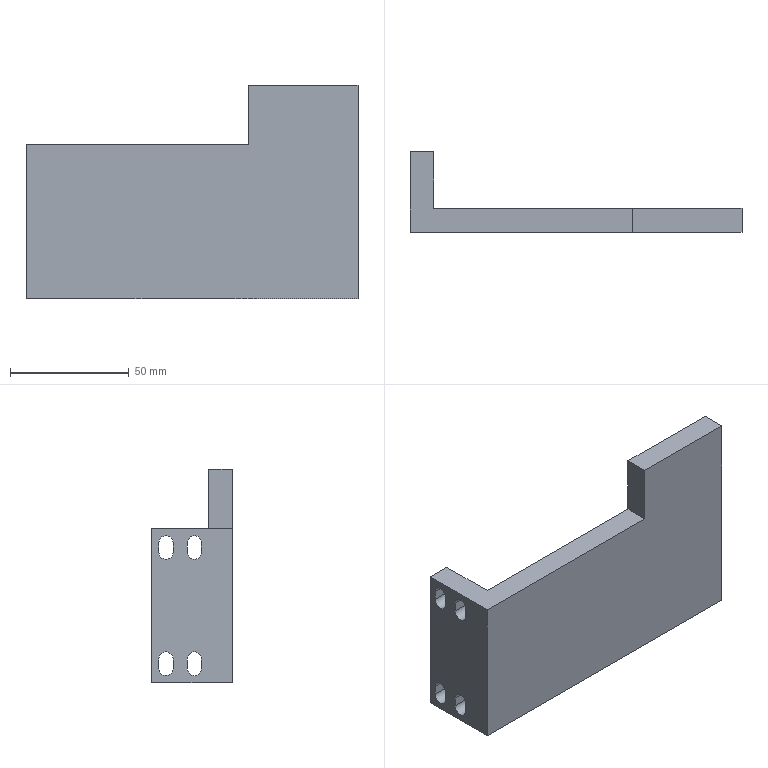Part | SolidWorks | features ICE 2, Extrusion 1 | 1 solid | 26 faces | box 140 x 34 x 90 mm | volume 116009 mm3 | plane 18 | cylinder 8 | commonest cylinder face diameters 6 x8
STEP:
#1=CARTESIAN_POINT('',(0.,0.,-32.5));
#2=VERTEX_POINT('',#1);
#3=CARTESIAN_POINT('',(140.,0.,-32.5));
#4=VERTEX_POINT('',#3);
#5=CARTESIAN_POINT('',(140.,0.,-32.5));
#6=DIRECTION('',(1.,0.,0.));
#7=VECTOR('',#6,1000.);
#8=LINE('',#5,#7);
#9=EDGE_CURVE('',#2,#4,#8,.T.);
#10=ORIENTED_EDGE('',*,*,#9,.T.);
#11=CARTESIAN_POINT('',(140.,0.,57.5));
#12=VERTEX_POINT('',#11);
#13=CARTESIAN_POINT('',(140.,0.,32.5));
#14=DIRECTION('',(0.,0.,-1.));
#15=VECTOR('',#14,1000.);
#16=LINE('',#13,#15);
#17=EDGE_CURVE('',#12,#4,#16,.T.);
#18=ORIENTED_EDGE('',*,*,#17,.F.);
#19=CARTESIAN_POINT('',(94.,0.,57.5));
#20=VERTEX_POINT('',#19);
#21=CARTESIAN_POINT('',(140.,0.,57.5));
#22=DIRECTION('',(-1.,0.,0.));
#23=VECTOR('',#22,1000.);
#24=LINE('',#21,#23);
#25=EDGE_CURVE('',#12,#20,#24,.T.);
#26=ORIENTED_EDGE('',*,*,#25,.T.);
#27=CARTESIAN_POINT('',(94.,0.,32.5));
#28=VERTEX_POINT('',#27);
#29=CARTESIAN_POINT('',(94.,0.,57.5));
#30=DIRECTION('',(0.,0.,-1.));
#31=VECTOR('',#30,1000.);
#32=LINE('',#29,#31);
#33=EDGE_CURVE('',#20,#28,#32,.T.);
#34=ORIENTED_EDGE('',*,*,#33,.T.);
#35=CARTESIAN_POINT('',(0.,0.,32.5));
#36=VERTEX_POINT('',#35);
#37=CARTESIAN_POINT('',(140.,0.,32.5));
#38=DIRECTION('',(1.,0.,0.));
#39=VECTOR('',#38,1000.);
#40=LINE('',#37,#39);
#41=EDGE_CURVE('',#36,#28,#40,.T.);
#42=ORIENTED_EDGE('',*,*,#41,.F.);
#43=CARTESIAN_POINT('',(0.,0.,32.5));
#44=DIRECTION('',(0.,0.,-1.));
#45=VECTOR('',#44,1000.);
#46=LINE('',#43,#45);
#47=EDGE_CURVE('',#36,#2,#46,.T.);
#48=ORIENTED_EDGE('',*,*,#47,.T.);
#49=EDGE_LOOP('',(#10,#18,#26,#34,#42,#48));
#50=FACE_OUTER_BOUND('',#49,.T.);
#51=CARTESIAN_POINT('',(140.,0.,32.5));
#52=DIRECTION('',(0.,1.,0.));
#53=DIRECTION('',(-1.,0.,0.));
#54=AXIS2_PLACEMENT_3D('',#51,#52,#53);
#55=PLANE('',#54);
#56=ADVANCED_FACE('',(#50),#55,.F.);
#57=CARTESIAN_POINT('',(140.,10.,-32.5));
#58=VERTEX_POINT('',#57);
#59=CARTESIAN_POINT('',(140.,10.,-32.5));
#60=DIRECTION('',(0.,1.,0.));
#61=VECTOR('',#60,1000.);
#62=LINE('',#59,#61);
#63=EDGE_CURVE('',#4,#58,#62,.T.);
#64=ORIENTED_EDGE('',*,*,#63,.T.);
#65=CARTESIAN_POINT('',(140.,10.,57.5));
#66=VERTEX_POINT('',#65);
#67=CARTESIAN_POINT('',(140.,10.,32.5));
#68=DIRECTION('',(0.,0.,-1.));
#69=VECTOR('',#68,1000.);
#70=LINE('',#67,#69);
#71=EDGE_CURVE('',#66,#58,#70,.T.);
#72=ORIENTED_EDGE('',*,*,#71,.F.);
#73=CARTESIAN_POINT('',(140.,-52.355,57.5));
#74=DIRECTION('',(0.,1.,0.));
#75=VECTOR('',#74,1000.);
#76=LINE('',#73,#75);
#77=EDGE_CURVE('',#12,#66,#76,.T.);
#78=ORIENTED_EDGE('',*,*,#77,.F.);
#79=ORIENTED_EDGE('',*,*,#17,.T.);
#80=EDGE_LOOP('',(#64,#72,#78,#79));
#81=FACE_OUTER_BOUND('',#80,.T.);
#82=CARTESIAN_POINT('',(140.,10.,32.5));
#83=DIRECTION('',(-1.,0.,0.));
#84=DIRECTION('',(0.,0.,1.));
#85=AXIS2_PLACEMENT_3D('',#82,#83,#84);
#86=PLANE('',#85);
#87=ADVANCED_FACE('',(#81),#86,.F.);
#88=CARTESIAN_POINT('',(10.,10.,-32.5));
#89=VERTEX_POINT('',#88);
#90=CARTESIAN_POINT('',(10.,10.,-32.5));
#91=DIRECTION('',(-1.,0.,0.));
#92=VECTOR('',#91,1000.);
#93=LINE('',#90,#92);
#94=EDGE_CURVE('',#58,#89,#93,.T.);
#95=ORIENTED_EDGE('',*,*,#94,.T.);
#96=CARTESIAN_POINT('',(10.,10.,32.5));
#97=VERTEX_POINT('',#96);
#98=CARTESIAN_POINT('',(10.,10.,32.5));
#99=DIRECTION('',(0.,0.,-1.));
#100=VECTOR('',#99,1000.);
#101=LINE('',#98,#100);
#102=EDGE_CURVE('',#97,#89,#101,.T.);
#103=ORIENTED_EDGE('',*,*,#102,.F.);
#104=CARTESIAN_POINT('',(94.,10.,32.5));
#105=VERTEX_POINT('',#104);
#106=CARTESIAN_POINT('',(10.,10.,32.5));
#107=DIRECTION('',(-1.,0.,0.));
#108=VECTOR('',#107,1000.);
#109=LINE('',#106,#108);
#110=EDGE_CURVE('',#105,#97,#109,.T.);
#111=ORIENTED_EDGE('',*,*,#110,.F.);
#112=CARTESIAN_POINT('',(94.,10.,57.5));
#113=VERTEX_POINT('',#112);
#114=CARTESIAN_POINT('',(94.,10.,57.5));
#115=DIRECTION('',(0.,0.,1.));
#116=VECTOR('',#115,1000.);
#117=LINE('',#114,#116);
#118=EDGE_CURVE('',#105,#113,#117,.T.);
#119=ORIENTED_EDGE('',*,*,#118,.T.);
#120=CARTESIAN_POINT('',(140.,10.,57.5));
#121=DIRECTION('',(1.,0.,0.));
#122=VECTOR('',#121,1000.);
#123=LINE('',#120,#122);
#124=EDGE_CURVE('',#113,#66,#123,.T.);
#125=ORIENTED_EDGE('',*,*,#124,.T.);
#126=ORIENTED_EDGE('',*,*,#71,.T.);
#127=EDGE_LOOP('',(#95,#103,#111,#119,#125,#126));
#128=FACE_OUTER_BOUND('',#127,.T.);
#129=CARTESIAN_POINT('',(10.,10.,32.5));
#130=DIRECTION('',(0.,-1.,0.));
#131=DIRECTION('',(1.,0.,0.));
#132=AXIS2_PLACEMENT_3D('',#129,#130,#131);
#133=PLANE('',#132);
#134=ADVANCED_FACE('',(#128),#133,.F.);
#135=CARTESIAN_POINT('',(10.,25.,-22.5));
#136=VERTEX_POINT('',#135);
#137=CARTESIAN_POINT('',(10.,25.,-26.5));
#138=VERTEX_POINT('',#137);
#139=CARTESIAN_POINT('',(10.,25.,-22.5));
#140=DIRECTION('',(0.,0.,-1.));
#141=VECTOR('',#140,1000.);
#142=LINE('',#139,#141);
#143=EDGE_CURVE('',#136,#138,#142,.T.);
#144=ORIENTED_EDGE('',*,*,#143,.F.);
#145=CARTESIAN_POINT('',(10.,31.,-22.5));
#146=VERTEX_POINT('',#145);
#147=CARTESIAN_POINT('',(10.,28.,-22.5));
#148=DIRECTION('',(1.,0.,0.));
#149=DIRECTION('',(0.,1.,0.));
#150=AXIS2_PLACEMENT_3D('',#147,#148,#149);
#151=CIRCLE('',#150,3.);
#152=EDGE_CURVE('',#146,#136,#151,.T.);
#153=ORIENTED_EDGE('',*,*,#152,.F.);
#154=CARTESIAN_POINT('',(10.,31.,-26.5));
#155=VERTEX_POINT('',#154);
#156=CARTESIAN_POINT('',(10.,31.,-22.5));
#157=DIRECTION('',(0.,0.,1.));
#158=VECTOR('',#157,1000.);
#159=LINE('',#156,#158);
#160=EDGE_CURVE('',#155,#146,#159,.T.);
#161=ORIENTED_EDGE('',*,*,#160,.F.);
#162=CARTESIAN_POINT('',(10.,28.,-26.5));
#163=DIRECTION('',(1.,0.,0.));
#164=DIRECTION('',(0.,1.,0.));
#165=AXIS2_PLACEMENT_3D('',#162,#163,#164);
#166=CIRCLE('',#165,3.);
#167=EDGE_CURVE('',#138,#155,#166,.T.);
#168=ORIENTED_EDGE('',*,*,#167,.F.);
#169=EDGE_LOOP('',(#144,#153,#161,#168));
#170=FACE_BOUND('',#169,.T.);
#171=CARTESIAN_POINT('',(10.,13.,26.5));
#172=VERTEX_POINT('',#171);
#173=CARTESIAN_POINT('',(10.,13.,22.5));
#174=VERTEX_POINT('',#173);
#175=CARTESIAN_POINT('',(10.,13.,26.5));
#176=DIRECTION('',(0.,0.,-1.));
#177=VECTOR('',#176,1000.);
#178=LINE('',#175,#177);
#179=EDGE_CURVE('',#172,#174,#178,.T.);
#180=ORIENTED_EDGE('',*,*,#179,.F.);
#181=CARTESIAN_POINT('',(10.,19.,26.5));
#182=VERTEX_POINT('',#181);
#183=CARTESIAN_POINT('',(10.,16.,26.5));
#184=DIRECTION('',(1.,0.,0.));
#185=DIRECTION('',(0.,-1.,0.));
#186=AXIS2_PLACEMENT_3D('',#183,#184,#185);
#187=CIRCLE('',#186,3.);
#188=EDGE_CURVE('',#182,#172,#187,.T.);
#189=ORIENTED_EDGE('',*,*,#188,.F.);
#190=CARTESIAN_POINT('',(10.,19.,22.5));
#191=VERTEX_POINT('',#190);
#192=CARTESIAN_POINT('',(10.,19.,26.5));
#193=DIRECTION('',(0.,0.,1.));
#194=VECTOR('',#193,1000.);
#195=LINE('',#192,#194);
#196=EDGE_CURVE('',#191,#182,#195,.T.);
#197=ORIENTED_EDGE('',*,*,#196,.F.);
#198=CARTESIAN_POINT('',(10.,16.,22.5));
#199=DIRECTION('',(1.,0.,0.));
#200=DIRECTION('',(0.,-1.,0.));
#201=AXIS2_PLACEMENT_3D('',#198,#199,#200);
#202=CIRCLE('',#201,3.);
#203=EDGE_CURVE('',#174,#191,#202,.T.);
#204=ORIENTED_EDGE('',*,*,#203,.F.);
#205=EDGE_LOOP('',(#180,#189,#197,#204));
#206=FACE_BOUND('',#205,.T.);
#207=CARTESIAN_POINT('',(10.,13.,-22.5));
#208=VERTEX_POINT('',#207);
#209=CARTESIAN_POINT('',(10.,13.,-26.5));
#210=VERTEX_POINT('',#209);
#211=CARTESIAN_POINT('',(10.,13.,-22.5));
#212=DIRECTION('',(0.,0.,-1.));
#213=VECTOR('',#212,1000.);
#214=LINE('',#211,#213);
#215=EDGE_CURVE('',#208,#210,#214,.T.);
#216=ORIENTED_EDGE('',*,*,#215,.F.);
#217=CARTESIAN_POINT('',(10.,19.,-22.5));
#218=VERTEX_POINT('',#217);
#219=CARTESIAN_POINT('',(10.,16.,-22.5));
#220=DIRECTION('',(1.,0.,0.));
#221=DIRECTION('',(0.,-1.,0.));
#222=AXIS2_PLACEMENT_3D('',#219,#220,#221);
#223=CIRCLE('',#222,3.);
#224=EDGE_CURVE('',#218,#208,#223,.T.);
#225=ORIENTED_EDGE('',*,*,#224,.F.);
#226=CARTESIAN_POINT('',(10.,19.,-26.5));
#227=VERTEX_POINT('',#226);
#228=CARTESIAN_POINT('',(10.,19.,-22.5));
#229=DIRECTION('',(0.,0.,1.));
#230=VECTOR('',#229,1000.);
#231=LINE('',#228,#230);
#232=EDGE_CURVE('',#227,#218,#231,.T.);
#233=ORIENTED_EDGE('',*,*,#232,.F.);
#234=CARTESIAN_POINT('',(10.,16.,-26.5));
#235=DIRECTION('',(1.,0.,0.));
#236=DIRECTION('',(0.,-1.,0.));
#237=AXIS2_PLACEMENT_3D('',#234,#235,#236);
#238=CIRCLE('',#237,3.);
#239=EDGE_CURVE('',#210,#227,#238,.T.);
#240=ORIENTED_EDGE('',*,*,#239,.F.);
#241=EDGE_LOOP('',(#216,#225,#233,#240));
#242=FACE_BOUND('',#241,.T.);
#243=CARTESIAN_POINT('',(10.,25.,26.5));
#244=VERTEX_POINT('',#243);
#245=CARTESIAN_POINT('',(10.,25.,22.5));
#246=VERTEX_POINT('',#245);
#247=CARTESIAN_POINT('',(10.,25.,26.5));
#248=DIRECTION('',(0.,0.,-1.));
#249=VECTOR('',#248,1000.);
#250=LINE('',#247,#249);
#251=EDGE_CURVE('',#244,#246,#250,.T.);
#252=ORIENTED_EDGE('',*,*,#251,.F.);
#253=CARTESIAN_POINT('',(10.,31.,26.5));
#254=VERTEX_POINT('',#253);
#255=CARTESIAN_POINT('',(10.,28.,26.5));
#256=DIRECTION('',(1.,0.,0.));
#257=DIRECTION('',(0.,1.,0.));
#258=AXIS2_PLACEMENT_3D('',#255,#256,#257);
#259=CIRCLE('',#258,3.);
#260=EDGE_CURVE('',#254,#244,#259,.T.);
#261=ORIENTED_EDGE('',*,*,#260,.F.);
#262=CARTESIAN_POINT('',(10.,31.,22.5));
#263=VERTEX_POINT('',#262);
#264=CARTESIAN_POINT('',(10.,31.,26.5));
#265=DIRECTION('',(0.,0.,1.));
#266=VECTOR('',#265,1000.);
#267=LINE('',#264,#266);
#268=EDGE_CURVE('',#263,#254,#267,.T.);
#269=ORIENTED_EDGE('',*,*,#268,.F.);
#270=CARTESIAN_POINT('',(10.,28.,22.5));
#271=DIRECTION('',(1.,0.,0.));
#272=DIRECTION('',(0.,1.,0.));
#273=AXIS2_PLACEMENT_3D('',#270,#271,#272);
#274=CIRCLE('',#273,3.);
#275=EDGE_CURVE('',#246,#263,#274,.T.);
#276=ORIENTED_EDGE('',*,*,#275,.F.);
#277=EDGE_LOOP('',(#252,#261,#269,#276));
#278=FACE_BOUND('',#277,.T.);
#279=CARTESIAN_POINT('',(10.,34.,-32.5));
#280=VERTEX_POINT('',#279);
#281=CARTESIAN_POINT('',(10.,34.,-32.5));
#282=DIRECTION('',(0.,1.,0.));
#283=VECTOR('',#282,1000.);
#284=LINE('',#281,#283);
#285=EDGE_CURVE('',#89,#280,#284,.T.);
#286=ORIENTED_EDGE('',*,*,#285,.T.);
#287=CARTESIAN_POINT('',(10.,34.,32.5));
#288=VERTEX_POINT('',#287);
#289=CARTESIAN_POINT('',(10.,34.,32.5));
#290=DIRECTION('',(0.,0.,-1.));
#291=VECTOR('',#290,1000.);
#292=LINE('',#289,#291);
#293=EDGE_CURVE('',#288,#280,#292,.T.);
#294=ORIENTED_EDGE('',*,*,#293,.F.);
#295=CARTESIAN_POINT('',(10.,34.,32.5));
#296=DIRECTION('',(0.,1.,0.));
#297=VECTOR('',#296,1000.);
#298=LINE('',#295,#297);
#299=EDGE_CURVE('',#97,#288,#298,.T.);
#300=ORIENTED_EDGE('',*,*,#299,.F.);
#301=ORIENTED_EDGE('',*,*,#102,.T.);
#302=EDGE_LOOP('',(#286,#294,#300,#301));
#303=FACE_OUTER_BOUND('',#302,.T.);
#304=CARTESIAN_POINT('',(10.,34.,32.5));
#305=DIRECTION('',(-1.,0.,0.));
#306=DIRECTION('',(0.,-1.,0.));
#307=AXIS2_PLACEMENT_3D('',#304,#305,#306);
#308=PLANE('',#307);
#309=ADVANCED_FACE('',(#170,#206,#242,#278,#303),#308,.F.);
#310=CARTESIAN_POINT('',(0.,34.,-32.5));
#311=VERTEX_POINT('',#310);
#312=CARTESIAN_POINT('',(0.,34.,-32.5));
#313=DIRECTION('',(-1.,0.,0.));
#314=VECTOR('',#313,1000.);
#315=LINE('',#312,#314);
#316=EDGE_CURVE('',#280,#311,#315,.T.);
#317=ORIENTED_EDGE('',*,*,#316,.T.);
#318=CARTESIAN_POINT('',(0.,34.,32.5));
#319=VERTEX_POINT('',#318);
#320=CARTESIAN_POINT('',(0.,34.,32.5));
#321=DIRECTION('',(0.,0.,-1.));
#322=VECTOR('',#321,1000.);
#323=LINE('',#320,#322);
#324=EDGE_CURVE('',#319,#311,#323,.T.);
#325=ORIENTED_EDGE('',*,*,#324,.F.);
#326=CARTESIAN_POINT('',(0.,34.,32.5));
#327=DIRECTION('',(-1.,0.,0.));
#328=VECTOR('',#327,1000.);
#329=LINE('',#326,#328);
#330=EDGE_CURVE('',#288,#319,#329,.T.);
#331=ORIENTED_EDGE('',*,*,#330,.F.);
#332=ORIENTED_EDGE('',*,*,#293,.T.);
#333=EDGE_LOOP('',(#317,#325,#331,#332));
#334=FACE_OUTER_BOUND('',#333,.T.);
#335=CARTESIAN_POINT('',(0.,34.,32.5));
#336=DIRECTION('',(0.,-1.,0.));
#337=DIRECTION('',(0.,0.,-1.));
#338=AXIS2_PLACEMENT_3D('',#335,#336,#337);
#339=PLANE('',#338);
#340=ADVANCED_FACE('',(#334),#339,.F.);
#341=CARTESIAN_POINT('',(0.,31.,-22.5));
#342=VERTEX_POINT('',#341);
#343=CARTESIAN_POINT('',(0.,31.,-26.5));
#344=VERTEX_POINT('',#343);
#345=CARTESIAN_POINT('',(0.,31.,-22.5));
#346=DIRECTION('',(0.,0.,-1.));
#347=VECTOR('',#346,1000.);
#348=LINE('',#345,#347);
#349=EDGE_CURVE('',#342,#344,#348,.T.);
#350=ORIENTED_EDGE('',*,*,#349,.F.);
#351=CARTESIAN_POINT('',(0.,25.,-22.5));
#352=VERTEX_POINT('',#351);
#353=CARTESIAN_POINT('',(0.,28.,-22.5));
#354=DIRECTION('',(-1.,0.,0.));
#355=DIRECTION('',(0.,1.,0.));
#356=AXIS2_PLACEMENT_3D('',#353,#354,#355);
#357=CIRCLE('',#356,3.);
#358=EDGE_CURVE('',#352,#342,#357,.T.);
#359=ORIENTED_EDGE('',*,*,#358,.F.);
#360=CARTESIAN_POINT('',(0.,25.,-26.5));
#361=VERTEX_POINT('',#360);
#362=CARTESIAN_POINT('',(0.,25.,-22.5));
#363=DIRECTION('',(0.,0.,1.));
#364=VECTOR('',#363,1000.);
#365=LINE('',#362,#364);
#366=EDGE_CURVE('',#361,#352,#365,.T.);
#367=ORIENTED_EDGE('',*,*,#366,.F.);
#368=CARTESIAN_POINT('',(0.,28.,-26.5));
#369=DIRECTION('',(-1.,0.,0.));
#370=DIRECTION('',(0.,1.,0.));
#371=AXIS2_PLACEMENT_3D('',#368,#369,#370);
#372=CIRCLE('',#371,3.);
#373=EDGE_CURVE('',#344,#361,#372,.T.);
#374=ORIENTED_EDGE('',*,*,#373,.F.);
#375=EDGE_LOOP('',(#350,#359,#367,#374));
#376=FACE_BOUND('',#375,.T.);
#377=CARTESIAN_POINT('',(0.,19.,26.5));
#378=VERTEX_POINT('',#377);
#379=CARTESIAN_POINT('',(0.,19.,22.5));
#380=VERTEX_POINT('',#379);
#381=CARTESIAN_POINT('',(0.,19.,26.5));
#382=DIRECTION('',(0.,0.,-1.));
#383=VECTOR('',#382,1000.);
#384=LINE('',#381,#383);
#385=EDGE_CURVE('',#378,#380,#384,.T.);
#386=ORIENTED_EDGE('',*,*,#385,.F.);
#387=CARTESIAN_POINT('',(0.,13.,26.5));
#388=VERTEX_POINT('',#387);
#389=CARTESIAN_POINT('',(0.,16.,26.5));
#390=DIRECTION('',(-1.,0.,0.));
#391=DIRECTION('',(0.,1.,0.));
#392=AXIS2_PLACEMENT_3D('',#389,#390,#391);
#393=CIRCLE('',#392,3.);
#394=EDGE_CURVE('',#388,#378,#393,.T.);
#395=ORIENTED_EDGE('',*,*,#394,.F.);
#396=CARTESIAN_POINT('',(0.,13.,22.5));
#397=VERTEX_POINT('',#396);
#398=CARTESIAN_POINT('',(0.,13.,26.5));
#399=DIRECTION('',(0.,0.,1.));
#400=VECTOR('',#399,1000.);
#401=LINE('',#398,#400);
#402=EDGE_CURVE('',#397,#388,#401,.T.);
#403=ORIENTED_EDGE('',*,*,#402,.F.);
#404=CARTESIAN_POINT('',(0.,16.,22.5));
#405=DIRECTION('',(-1.,0.,0.));
#406=DIRECTION('',(0.,1.,0.));
#407=AXIS2_PLACEMENT_3D('',#404,#405,#406);
#408=CIRCLE('',#407,3.);
#409=EDGE_CURVE('',#380,#397,#408,.T.);
#410=ORIENTED_EDGE('',*,*,#409,.F.);
#411=EDGE_LOOP('',(#386,#395,#403,#410));
#412=FACE_BOUND('',#411,.T.);
#413=CARTESIAN_POINT('',(0.,19.,-22.5));
#414=VERTEX_POINT('',#413);
#415=CARTESIAN_POINT('',(0.,19.,-26.5));
#416=VERTEX_POINT('',#415);
#417=CARTESIAN_POINT('',(0.,19.,-22.5));
#418=DIRECTION('',(0.,0.,-1.));
#419=VECTOR('',#418,1000.);
#420=LINE('',#417,#419);
#421=EDGE_CURVE('',#414,#416,#420,.T.);
#422=ORIENTED_EDGE('',*,*,#421,.F.);
#423=CARTESIAN_POINT('',(0.,13.,-22.5));
#424=VERTEX_POINT('',#423);
#425=CARTESIAN_POINT('',(0.,16.,-22.5));
#426=DIRECTION('',(-1.,0.,0.));
#427=DIRECTION('',(0.,1.,0.));
#428=AXIS2_PLACEMENT_3D('',#425,#426,#427);
#429=CIRCLE('',#428,3.);
#430=EDGE_CURVE('',#424,#414,#429,.T.);
#431=ORIENTED_EDGE('',*,*,#430,.F.);
#432=CARTESIAN_POINT('',(0.,13.,-26.5));
#433=VERTEX_POINT('',#432);
#434=CARTESIAN_POINT('',(0.,13.,-22.5));
#435=DIRECTION('',(0.,0.,1.));
#436=VECTOR('',#435,1000.);
#437=LINE('',#434,#436);
#438=EDGE_CURVE('',#433,#424,#437,.T.);
#439=ORIENTED_EDGE('',*,*,#438,.F.);
#440=CARTESIAN_POINT('',(0.,16.,-26.5));
#441=DIRECTION('',(-1.,0.,0.));
#442=DIRECTION('',(0.,1.,0.));
#443=AXIS2_PLACEMENT_3D('',#440,#441,#442);
#444=CIRCLE('',#443,3.);
#445=EDGE_CURVE('',#416,#433,#444,.T.);
#446=ORIENTED_EDGE('',*,*,#445,.F.);
#447=EDGE_LOOP('',(#422,#431,#439,#446));
#448=FACE_BOUND('',#447,.T.);
#449=CARTESIAN_POINT('',(0.,31.,26.5));
#450=VERTEX_POINT('',#449);
#451=CARTESIAN_POINT('',(0.,31.,22.5));
#452=VERTEX_POINT('',#451);
#453=CARTESIAN_POINT('',(0.,31.,26.5));
#454=DIRECTION('',(0.,0.,-1.));
#455=VECTOR('',#454,1000.);
#456=LINE('',#453,#455);
#457=EDGE_CURVE('',#450,#452,#456,.T.);
#458=ORIENTED_EDGE('',*,*,#457,.F.);
#459=CARTESIAN_POINT('',(0.,25.,26.5));
#460=VERTEX_POINT('',#459);
#461=CARTESIAN_POINT('',(0.,28.,26.5));
#462=DIRECTION('',(-1.,0.,0.));
#463=DIRECTION('',(0.,1.,0.));
#464=AXIS2_PLACEMENT_3D('',#461,#462,#463);
#465=CIRCLE('',#464,3.);
#466=EDGE_CURVE('',#460,#450,#465,.T.);
#467=ORIENTED_EDGE('',*,*,#466,.F.);
#468=CARTESIAN_POINT('',(0.,25.,22.5));
#469=VERTEX_POINT('',#468);
#470=CARTESIAN_POINT('',(0.,25.,26.5));
#471=DIRECTION('',(0.,0.,1.));
#472=VECTOR('',#471,1000.);
#473=LINE('',#470,#472);
#474=EDGE_CURVE('',#469,#460,#473,.T.);
#475=ORIENTED_EDGE('',*,*,#474,.F.);
#476=CARTESIAN_POINT('',(0.,28.,22.5));
#477=DIRECTION('',(-1.,0.,0.));
#478=DIRECTION('',(0.,1.,0.));
#479=AXIS2_PLACEMENT_3D('',#476,#477,#478);
#480=CIRCLE('',#479,3.);
#481=EDGE_CURVE('',#452,#469,#480,.T.);
#482=ORIENTED_EDGE('',*,*,#481,.F.);
#483=EDGE_LOOP('',(#458,#467,#475,#482));
#484=FACE_BOUND('',#483,.T.);
#485=CARTESIAN_POINT('',(0.,0.,-32.5));
#486=DIRECTION('',(0.,-1.,0.));
#487=VECTOR('',#486,1000.);
#488=LINE('',#485,#487);
#489=EDGE_CURVE('',#311,#2,#488,.T.);
#490=ORIENTED_EDGE('',*,*,#489,.T.);
#491=ORIENTED_EDGE('',*,*,#47,.F.);
#492=CARTESIAN_POINT('',(0.,0.,32.5));
#493=DIRECTION('',(0.,-1.,0.));
#494=VECTOR('',#493,1000.);
#495=LINE('',#492,#494);
#496=EDGE_CURVE('',#319,#36,#495,.T.);
#497=ORIENTED_EDGE('',*,*,#496,.F.);
#498=ORIENTED_EDGE('',*,*,#324,.T.);
#499=EDGE_LOOP('',(#490,#491,#497,#498));
#500=FACE_OUTER_BOUND('',#499,.T.);
#501=CARTESIAN_POINT('',(0.,0.,32.5));
#502=DIRECTION('',(1.,0.,0.));
#503=DIRECTION('',(0.,1.,0.));
#504=AXIS2_PLACEMENT_3D('',#501,#502,#503);
#505=PLANE('',#504);
#506=ADVANCED_FACE('',(#376,#412,#448,#484,#500),#505,.F.);
#507=ORIENTED_EDGE('',*,*,#41,.T.);
#508=CARTESIAN_POINT('',(94.,-52.355,32.5));
#509=DIRECTION('',(0.,1.,0.));
#510=VECTOR('',#509,1000.);
#511=LINE('',#508,#510);
#512=EDGE_CURVE('',#28,#105,#511,.T.);
#513=ORIENTED_EDGE('',*,*,#512,.T.);
#514=ORIENTED_EDGE('',*,*,#110,.T.);
#515=ORIENTED_EDGE('',*,*,#299,.T.);
#516=ORIENTED_EDGE('',*,*,#330,.T.);
#517=ORIENTED_EDGE('',*,*,#496,.T.);
#518=EDGE_LOOP('',(#507,#513,#514,#515,#516,#517));
#519=FACE_OUTER_BOUND('',#518,.T.);
#520=CARTESIAN_POINT('',(0.,0.,32.5));
#521=DIRECTION('',(0.,0.,-1.));
#522=DIRECTION('',(-1.,0.,0.));
#523=AXIS2_PLACEMENT_3D('',#520,#521,#522);
#524=PLANE('',#523);
#525=ADVANCED_FACE('',(#519),#524,.F.);
#526=ORIENTED_EDGE('',*,*,#9,.F.);
#527=ORIENTED_EDGE('',*,*,#489,.F.);
#528=ORIENTED_EDGE('',*,*,#316,.F.);
#529=ORIENTED_EDGE('',*,*,#285,.F.);
#530=ORIENTED_EDGE('',*,*,#94,.F.);
#531=ORIENTED_EDGE('',*,*,#63,.F.);
#532=EDGE_LOOP('',(#526,#527,#528,#529,#530,#531));
#533=FACE_OUTER_BOUND('',#532,.T.);
#534=CARTESIAN_POINT('',(0.,0.,-32.5));
#535=DIRECTION('',(0.,0.,-1.));
#536=DIRECTION('',(-1.,0.,0.));
#537=AXIS2_PLACEMENT_3D('',#534,#535,#536);
#538=PLANE('',#537);
#539=ADVANCED_FACE('',(#533),#538,.T.);
#540=ORIENTED_EDGE('',*,*,#466,.T.);
#541=CARTESIAN_POINT('',(-0.001,31.,26.5));
#542=DIRECTION('',(1.,0.,0.));
#543=VECTOR('',#542,1000.);
#544=LINE('',#541,#543);
#545=EDGE_CURVE('',#450,#254,#544,.T.);
#546=ORIENTED_EDGE('',*,*,#545,.T.);
#547=ORIENTED_EDGE('',*,*,#260,.T.);
#548=CARTESIAN_POINT('',(-0.001,25.,26.5));
#549=DIRECTION('',(1.,0.,0.));
#550=VECTOR('',#549,1000.);
#551=LINE('',#548,#550);
#552=EDGE_CURVE('',#460,#244,#551,.T.);
#553=ORIENTED_EDGE('',*,*,#552,.F.);
#554=EDGE_LOOP('',(#540,#546,#547,#553));
#555=FACE_OUTER_BOUND('',#554,.T.);
#556=CARTESIAN_POINT('',(-0.001,28.,26.5));
#557=DIRECTION('',(1.,0.,0.));
#558=DIRECTION('',(0.,1.,0.));
#559=AXIS2_PLACEMENT_3D('',#556,#557,#558);
#560=CYLINDRICAL_SURFACE('',#559,3.);
#561=ADVANCED_FACE('',(#555),#560,.F.);
#562=ORIENTED_EDGE('',*,*,#457,.T.);
#563=CARTESIAN_POINT('',(-0.001,31.,22.5));
#564=DIRECTION('',(1.,0.,0.));
#565=VECTOR('',#564,1000.);
#566=LINE('',#563,#565);
#567=EDGE_CURVE('',#452,#263,#566,.T.);
#568=ORIENTED_EDGE('',*,*,#567,.T.);
#569=ORIENTED_EDGE('',*,*,#268,.T.);
#570=ORIENTED_EDGE('',*,*,#545,.F.);
#571=EDGE_LOOP('',(#562,#568,#569,#570));
#572=FACE_OUTER_BOUND('',#571,.T.);
#573=CARTESIAN_POINT('',(-0.001,31.,26.5));
#574=DIRECTION('',(0.,1.,0.));
#575=DIRECTION('',(-1.,0.,0.));
#576=AXIS2_PLACEMENT_3D('',#573,#574,#575);
#577=PLANE('',#576);
#578=ADVANCED_FACE('',(#572),#577,.F.);
#579=ORIENTED_EDGE('',*,*,#481,.T.);
#580=CARTESIAN_POINT('',(-0.001,25.,22.5));
#581=DIRECTION('',(1.,0.,0.));
#582=VECTOR('',#581,1000.);
#583=LINE('',#580,#582);
#584=EDGE_CURVE('',#469,#246,#583,.T.);
#585=ORIENTED_EDGE('',*,*,#584,.T.);
#586=ORIENTED_EDGE('',*,*,#275,.T.);
#587=ORIENTED_EDGE('',*,*,#567,.F.);
#588=EDGE_LOOP('',(#579,#585,#586,#587));
#589=FACE_OUTER_BOUND('',#588,.T.);
#590=CARTESIAN_POINT('',(-0.001,28.,22.5));
#591=DIRECTION('',(1.,0.,0.));
#592=DIRECTION('',(0.,1.,0.));
#593=AXIS2_PLACEMENT_3D('',#590,#591,#592);
#594=CYLINDRICAL_SURFACE('',#593,3.);
#595=ADVANCED_FACE('',(#589),#594,.F.);
#596=ORIENTED_EDGE('',*,*,#474,.T.);
#597=ORIENTED_EDGE('',*,*,#552,.T.);
#598=ORIENTED_EDGE('',*,*,#251,.T.);
#599=ORIENTED_EDGE('',*,*,#584,.F.);
#600=EDGE_LOOP('',(#596,#597,#598,#599));
#601=FACE_OUTER_BOUND('',#600,.T.);
#602=CARTESIAN_POINT('',(-0.001,25.,26.5));
#603=DIRECTION('',(0.,-1.,0.));
#604=DIRECTION('',(1.,0.,0.));
#605=AXIS2_PLACEMENT_3D('',#602,#603,#604);
#606=PLANE('',#605);
#607=ADVANCED_FACE('',(#601),#606,.F.);
#608=ORIENTED_EDGE('',*,*,#430,.T.);
#609=CARTESIAN_POINT('',(-0.001,19.,-22.5));
#610=DIRECTION('',(1.,0.,0.));
#611=VECTOR('',#610,1000.);
#612=LINE('',#609,#611);
#613=EDGE_CURVE('',#414,#218,#612,.T.);
#614=ORIENTED_EDGE('',*,*,#613,.T.);
#615=ORIENTED_EDGE('',*,*,#224,.T.);
#616=CARTESIAN_POINT('',(-0.001,13.,-22.5));
#617=DIRECTION('',(1.,0.,0.));
#618=VECTOR('',#617,1000.);
#619=LINE('',#616,#618);
#620=EDGE_CURVE('',#424,#208,#619,.T.);
#621=ORIENTED_EDGE('',*,*,#620,.F.);
#622=EDGE_LOOP('',(#608,#614,#615,#621));
#623=FACE_OUTER_BOUND('',#622,.T.);
#624=CARTESIAN_POINT('',(-0.001,16.,-22.5));
#625=DIRECTION('',(1.,0.,0.));
#626=DIRECTION('',(0.,1.,0.));
#627=AXIS2_PLACEMENT_3D('',#624,#625,#626);
#628=CYLINDRICAL_SURFACE('',#627,3.);
#629=ADVANCED_FACE('',(#623),#628,.F.);
#630=ORIENTED_EDGE('',*,*,#421,.T.);
#631=CARTESIAN_POINT('',(-0.001,19.,-26.5));
#632=DIRECTION('',(1.,0.,0.));
#633=VECTOR('',#632,1000.);
#634=LINE('',#631,#633);
#635=EDGE_CURVE('',#416,#227,#634,.T.);
#636=ORIENTED_EDGE('',*,*,#635,.T.);
#637=ORIENTED_EDGE('',*,*,#232,.T.);
#638=ORIENTED_EDGE('',*,*,#613,.F.);
#639=EDGE_LOOP('',(#630,#636,#637,#638));
#640=FACE_OUTER_BOUND('',#639,.T.);
#641=CARTESIAN_POINT('',(-0.001,19.,-22.5));
#642=DIRECTION('',(0.,1.,0.));
#643=DIRECTION('',(-1.,0.,0.));
#644=AXIS2_PLACEMENT_3D('',#641,#642,#643);
#645=PLANE('',#644);
#646=ADVANCED_FACE('',(#640),#645,.F.);
#647=ORIENTED_EDGE('',*,*,#445,.T.);
#648=CARTESIAN_POINT('',(-0.001,13.,-26.5));
#649=DIRECTION('',(1.,0.,0.));
#650=VECTOR('',#649,1000.);
#651=LINE('',#648,#650);
#652=EDGE_CURVE('',#433,#210,#651,.T.);
#653=ORIENTED_EDGE('',*,*,#652,.T.);
#654=ORIENTED_EDGE('',*,*,#239,.T.);
#655=ORIENTED_EDGE('',*,*,#635,.F.);
#656=EDGE_LOOP('',(#647,#653,#654,#655));
#657=FACE_OUTER_BOUND('',#656,.T.);
#658=CARTESIAN_POINT('',(-0.001,16.,-26.5));
#659=DIRECTION('',(1.,0.,0.));
#660=DIRECTION('',(0.,1.,0.));
#661=AXIS2_PLACEMENT_3D('',#658,#659,#660);
#662=CYLINDRICAL_SURFACE('',#661,3.);
#663=ADVANCED_FACE('',(#657),#662,.F.);
#664=ORIENTED_EDGE('',*,*,#438,.T.);
#665=ORIENTED_EDGE('',*,*,#620,.T.);
#666=ORIENTED_EDGE('',*,*,#215,.T.);
#667=ORIENTED_EDGE('',*,*,#652,.F.);
#668=EDGE_LOOP('',(#664,#665,#666,#667));
#669=FACE_OUTER_BOUND('',#668,.T.);
#670=CARTESIAN_POINT('',(-0.001,13.,-22.5));
#671=DIRECTION('',(0.,-1.,0.));
#672=DIRECTION('',(1.,0.,0.));
#673=AXIS2_PLACEMENT_3D('',#670,#671,#672);
#674=PLANE('',#673);
#675=ADVANCED_FACE('',(#669),#674,.F.);
#676=ORIENTED_EDGE('',*,*,#394,.T.);
#677=CARTESIAN_POINT('',(-0.001,19.,26.5));
#678=DIRECTION('',(1.,0.,0.));
#679=VECTOR('',#678,1000.);
#680=LINE('',#677,#679);
#681=EDGE_CURVE('',#378,#182,#680,.T.);
#682=ORIENTED_EDGE('',*,*,#681,.T.);
#683=ORIENTED_EDGE('',*,*,#188,.T.);
#684=CARTESIAN_POINT('',(-0.001,13.,26.5));
#685=DIRECTION('',(1.,0.,0.));
#686=VECTOR('',#685,1000.);
#687=LINE('',#684,#686);
#688=EDGE_CURVE('',#388,#172,#687,.T.);
#689=ORIENTED_EDGE('',*,*,#688,.F.);
#690=EDGE_LOOP('',(#676,#682,#683,#689));
#691=FACE_OUTER_BOUND('',#690,.T.);
#692=CARTESIAN_POINT('',(-0.001,16.,26.5));
#693=DIRECTION('',(1.,0.,0.));
#694=DIRECTION('',(0.,1.,0.));
#695=AXIS2_PLACEMENT_3D('',#692,#693,#694);
#696=CYLINDRICAL_SURFACE('',#695,3.);
#697=ADVANCED_FACE('',(#691),#696,.F.);
#698=ORIENTED_EDGE('',*,*,#385,.T.);
#699=CARTESIAN_POINT('',(-0.001,19.,22.5));
#700=DIRECTION('',(1.,0.,0.));
#701=VECTOR('',#700,1000.);
#702=LINE('',#699,#701);
#703=EDGE_CURVE('',#380,#191,#702,.T.);
#704=ORIENTED_EDGE('',*,*,#703,.T.);
#705=ORIENTED_EDGE('',*,*,#196,.T.);
#706=ORIENTED_EDGE('',*,*,#681,.F.);
#707=EDGE_LOOP('',(#698,#704,#705,#706));
#708=FACE_OUTER_BOUND('',#707,.T.);
#709=CARTESIAN_POINT('',(-0.001,19.,26.5));
#710=DIRECTION('',(0.,1.,0.));
#711=DIRECTION('',(-1.,0.,0.));
#712=AXIS2_PLACEMENT_3D('',#709,#710,#711);
#713=PLANE('',#712);
#714=ADVANCED_FACE('',(#708),#713,.F.);
#715=ORIENTED_EDGE('',*,*,#409,.T.);
#716=CARTESIAN_POINT('',(-0.001,13.,22.5));
#717=DIRECTION('',(1.,0.,0.));
#718=VECTOR('',#717,1000.);
#719=LINE('',#716,#718);
#720=EDGE_CURVE('',#397,#174,#719,.T.);
#721=ORIENTED_EDGE('',*,*,#720,.T.);
#722=ORIENTED_EDGE('',*,*,#203,.T.);
#723=ORIENTED_EDGE('',*,*,#703,.F.);
#724=EDGE_LOOP('',(#715,#721,#722,#723));
#725=FACE_OUTER_BOUND('',#724,.T.);
#726=CARTESIAN_POINT('',(-0.001,16.,22.5));
#727=DIRECTION('',(1.,0.,0.));
#728=DIRECTION('',(0.,1.,0.));
#729=AXIS2_PLACEMENT_3D('',#726,#727,#728);
#730=CYLINDRICAL_SURFACE('',#729,3.);
#731=ADVANCED_FACE('',(#725),#730,.F.);
#732=ORIENTED_EDGE('',*,*,#402,.T.);
#733=ORIENTED_EDGE('',*,*,#688,.T.);
#734=ORIENTED_EDGE('',*,*,#179,.T.);
#735=ORIENTED_EDGE('',*,*,#720,.F.);
#736=EDGE_LOOP('',(#732,#733,#734,#735));
#737=FACE_OUTER_BOUND('',#736,.T.);
#738=CARTESIAN_POINT('',(-0.001,13.,26.5));
#739=DIRECTION('',(0.,-1.,0.));
#740=DIRECTION('',(1.,0.,0.));
#741=AXIS2_PLACEMENT_3D('',#738,#739,#740);
#742=PLANE('',#741);
#743=ADVANCED_FACE('',(#737),#742,.F.);
#744=ORIENTED_EDGE('',*,*,#358,.T.);
#745=CARTESIAN_POINT('',(-0.001,31.,-22.5));
#746=DIRECTION('',(1.,0.,0.));
#747=VECTOR('',#746,1000.);
#748=LINE('',#745,#747);
#749=EDGE_CURVE('',#342,#146,#748,.T.);
#750=ORIENTED_EDGE('',*,*,#749,.T.);
#751=ORIENTED_EDGE('',*,*,#152,.T.);
#752=CARTESIAN_POINT('',(-0.001,25.,-22.5));
#753=DIRECTION('',(1.,0.,0.));
#754=VECTOR('',#753,1000.);
#755=LINE('',#752,#754);
#756=EDGE_CURVE('',#352,#136,#755,.T.);
#757=ORIENTED_EDGE('',*,*,#756,.F.);
#758=EDGE_LOOP('',(#744,#750,#751,#757));
#759=FACE_OUTER_BOUND('',#758,.T.);
#760=CARTESIAN_POINT('',(-0.001,28.,-22.5));
#761=DIRECTION('',(1.,0.,0.));
#762=DIRECTION('',(0.,1.,0.));
#763=AXIS2_PLACEMENT_3D('',#760,#761,#762);
#764=CYLINDRICAL_SURFACE('',#763,3.);
#765=ADVANCED_FACE('',(#759),#764,.F.);
#766=ORIENTED_EDGE('',*,*,#349,.T.);
#767=CARTESIAN_POINT('',(-0.001,31.,-26.5));
#768=DIRECTION('',(1.,0.,0.));
#769=VECTOR('',#768,1000.);
#770=LINE('',#767,#769);
#771=EDGE_CURVE('',#344,#155,#770,.T.);
#772=ORIENTED_EDGE('',*,*,#771,.T.);
#773=ORIENTED_EDGE('',*,*,#160,.T.);
#774=ORIENTED_EDGE('',*,*,#749,.F.);
#775=EDGE_LOOP('',(#766,#772,#773,#774));
#776=FACE_OUTER_BOUND('',#775,.T.);
#777=CARTESIAN_POINT('',(-0.001,31.,-22.5));
#778=DIRECTION('',(0.,1.,0.));
#779=DIRECTION('',(-1.,0.,0.));
#780=AXIS2_PLACEMENT_3D('',#777,#778,#779);
#781=PLANE('',#780);
#782=ADVANCED_FACE('',(#776),#781,.F.);
#783=ORIENTED_EDGE('',*,*,#373,.T.);
#784=CARTESIAN_POINT('',(-0.001,25.,-26.5));
#785=DIRECTION('',(1.,0.,0.));
#786=VECTOR('',#785,1000.);
#787=LINE('',#784,#786);
#788=EDGE_CURVE('',#361,#138,#787,.T.);
#789=ORIENTED_EDGE('',*,*,#788,.T.);
#790=ORIENTED_EDGE('',*,*,#167,.T.);
#791=ORIENTED_EDGE('',*,*,#771,.F.);
#792=EDGE_LOOP('',(#783,#789,#790,#791));
#793=FACE_OUTER_BOUND('',#792,.T.);
#794=CARTESIAN_POINT('',(-0.001,28.,-26.5));
#795=DIRECTION('',(1.,0.,0.));
#796=DIRECTION('',(0.,1.,0.));
#797=AXIS2_PLACEMENT_3D('',#794,#795,#796);
#798=CYLINDRICAL_SURFACE('',#797,3.);
#799=ADVANCED_FACE('',(#793),#798,.F.);
#800=ORIENTED_EDGE('',*,*,#366,.T.);
#801=ORIENTED_EDGE('',*,*,#756,.T.);
#802=ORIENTED_EDGE('',*,*,#143,.T.);
#803=ORIENTED_EDGE('',*,*,#788,.F.);
#804=EDGE_LOOP('',(#800,#801,#802,#803));
#805=FACE_OUTER_BOUND('',#804,.T.);
#806=CARTESIAN_POINT('',(-0.001,25.,-22.5));
#807=DIRECTION('',(0.,-1.,0.));
#808=DIRECTION('',(1.,0.,0.));
#809=AXIS2_PLACEMENT_3D('',#806,#807,#808);
#810=PLANE('',#809);
#811=ADVANCED_FACE('',(#805),#810,.F.);
#812=ORIENTED_EDGE('',*,*,#25,.F.);
#813=ORIENTED_EDGE('',*,*,#77,.T.);
#814=ORIENTED_EDGE('',*,*,#124,.F.);
#815=CARTESIAN_POINT('',(94.,-52.355,57.5));
#816=DIRECTION('',(0.,1.,0.));
#817=VECTOR('',#816,1000.);
#818=LINE('',#815,#817);
#819=EDGE_CURVE('',#20,#113,#818,.T.);
#820=ORIENTED_EDGE('',*,*,#819,.F.);
#821=EDGE_LOOP('',(#812,#813,#814,#820));
#822=FACE_OUTER_BOUND('',#821,.T.);
#823=CARTESIAN_POINT('',(140.,-52.355,57.5));
#824=DIRECTION('',(0.,0.,1.));
#825=DIRECTION('',(1.,0.,0.));
#826=AXIS2_PLACEMENT_3D('',#823,#824,#825);
#827=PLANE('',#826);
#828=ADVANCED_FACE('',(#822),#827,.T.);
#829=ORIENTED_EDGE('',*,*,#33,.F.);
#830=ORIENTED_EDGE('',*,*,#819,.T.);
#831=ORIENTED_EDGE('',*,*,#118,.F.);
#832=ORIENTED_EDGE('',*,*,#512,.F.);
#833=EDGE_LOOP('',(#829,#830,#831,#832));
#834=FACE_OUTER_BOUND('',#833,.T.);
#835=CARTESIAN_POINT('',(94.,-52.355,57.5));
#836=DIRECTION('',(-1.,0.,0.));
#837=DIRECTION('',(0.,-1.,0.));
#838=AXIS2_PLACEMENT_3D('',#835,#836,#837);
#839=PLANE('',#838);
#840=ADVANCED_FACE('',(#834),#839,.T.);
#841=CLOSED_SHELL('',(#56,#87,#134,#309,#340,#506,#525,#539,#561,#578,#595,#607,#629,#646,#663,#675,#697,#714,#731,#743,#765,#782,#799,#811,#828,#840));
#842=MANIFOLD_SOLID_BREP('',#841);
#843=CARTESIAN_POINT('',(0.,0.,0.));
#844=DIRECTION('',(0.,0.,1.));
#845=DIRECTION('',(1.,0.,0.));
#846=AXIS2_PLACEMENT_3D('',#843,#844,#845);
#847=(LENGTH_UNIT()NAMED_UNIT(*)SI_UNIT(.MILLI.,.METRE.));
#848=UNCERTAINTY_MEASURE_WITH_UNIT(LENGTH_MEASURE(0.00001),#847,'','');
#849=(NAMED_UNIT(*)PLANE_ANGLE_UNIT()SI_UNIT($,.RADIAN.));
#850=(NAMED_UNIT(*)SI_UNIT($,.STERADIAN.)SOLID_ANGLE_UNIT());
#851=(GEOMETRIC_REPRESENTATION_CONTEXT(3)GLOBAL_UNCERTAINTY_ASSIGNED_CONTEXT((#848))GLOBAL_UNIT_ASSIGNED_CONTEXT((#847,#849,#850))REPRESENTATION_CONTEXT('',''));
#852=ADVANCED_BREP_SHAPE_REPRESENTATION('',(#842,#846),#851);